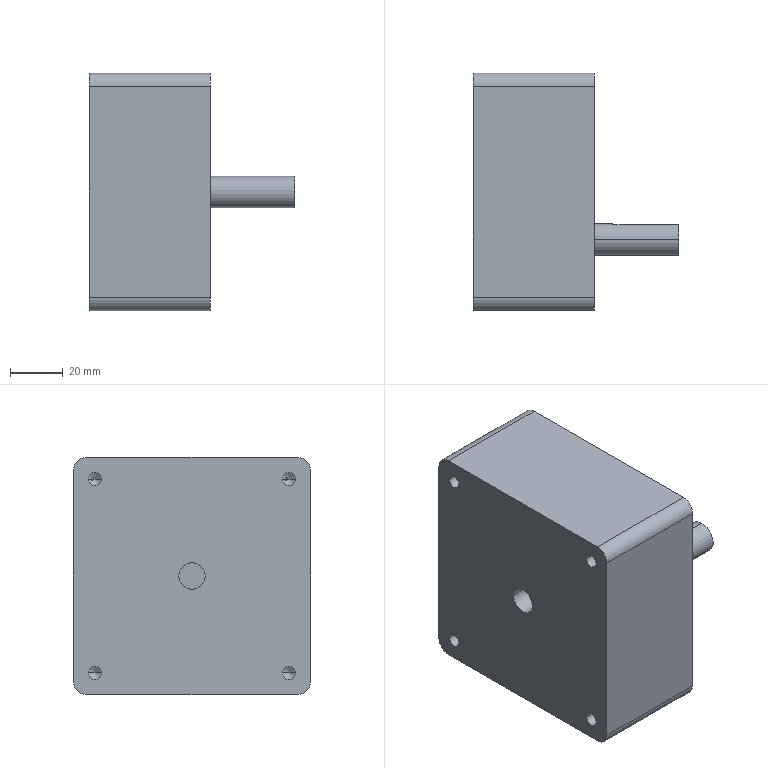Part | STEP file | 40W JSCC gear motor | 1 solid | 52 faces | box 78 x 90 x 90 mm | volume 369652 mm3 | cylinder 24 | cone 16 | plane 12 | commonest cylinder face diameters 5 x16 10 x6 12 x2